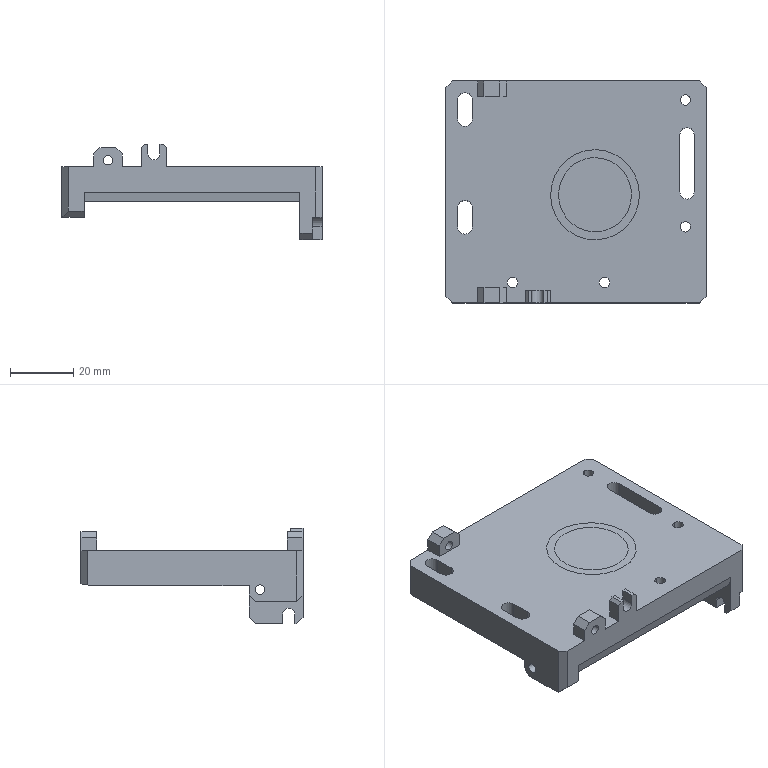Part | 2 solids | 113 faces | box 82 x 70 x 30 mm | volume 63316 mm3 | plane 64 | cylinder 41 | cone 8 | commonest cylinder face diameters 3 x8 3.3 x8 4.6 x6 2 x4 4.5 x3 28 x3